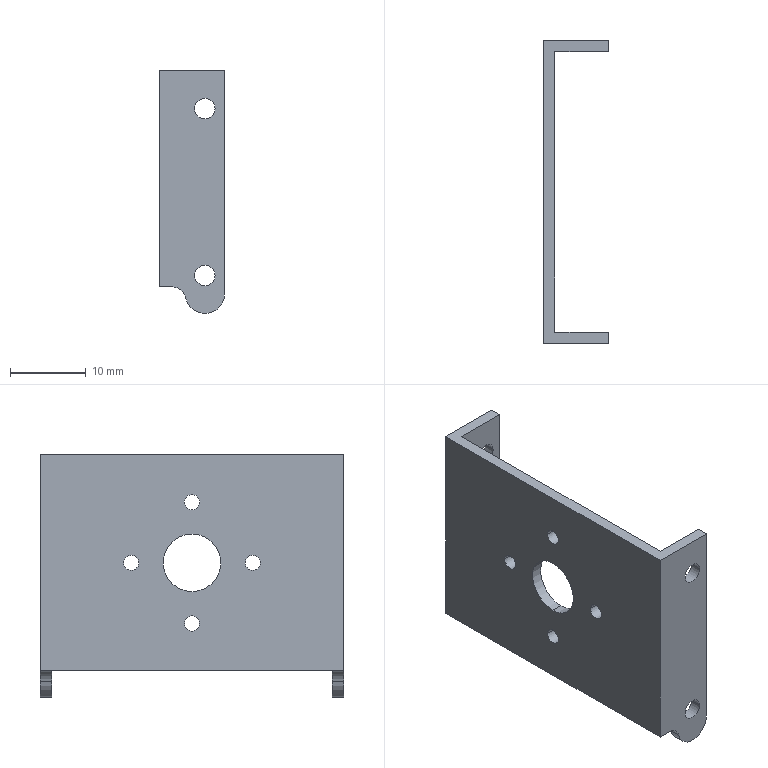Part | SolidWorks | features BaseBody 1 | 1 solid | 32 faces | box 8.6 x 40 x 32 mm | volume 2244 mm3 | cylinder 22 | plane 10 | commonest cylinder face diameters 2 x8 2.7 x8 3.485 x2 5.2 x2 7.6 x2
STEP:
#1=CARTESIAN_POINT('',(0.,19.,9.743));
#2=VERTEX_POINT('',#1);
#3=CARTESIAN_POINT('',(0.,21.,9.743));
#4=VERTEX_POINT('',#3);
#5=CARTESIAN_POINT('',(0.,20.,9.743));
#6=DIRECTION('',(1.,0.,0.));
#7=DIRECTION('',(0.,0.,1.));
#8=AXIS2_PLACEMENT_3D('',#5,#6,#7);
#9=CIRCLE('',#8,1.);
#10=EDGE_CURVE('',#2,#4,#9,.T.);
#11=ORIENTED_EDGE('',*,*,#10,.F.);
#12=CARTESIAN_POINT('',(1.5,19.,9.743));
#13=VERTEX_POINT('',#12);
#14=CARTESIAN_POINT('',(0.,19.,9.743));
#15=DIRECTION('',(1.,0.,0.));
#16=VECTOR('',#15,1000.);
#17=LINE('',#14,#16);
#18=EDGE_CURVE('',#2,#13,#17,.T.);
#19=ORIENTED_EDGE('',*,*,#18,.T.);
#20=CARTESIAN_POINT('',(1.5,21.,9.743));
#21=VERTEX_POINT('',#20);
#22=CARTESIAN_POINT('',(1.5,20.,9.743));
#23=DIRECTION('',(1.,0.,0.));
#24=DIRECTION('',(0.,0.,1.));
#25=AXIS2_PLACEMENT_3D('',#22,#23,#24);
#26=CIRCLE('',#25,1.);
#27=EDGE_CURVE('',#13,#21,#26,.T.);
#28=ORIENTED_EDGE('',*,*,#27,.T.);
#29=CARTESIAN_POINT('',(0.,21.,9.743));
#30=DIRECTION('',(1.,0.,0.));
#31=VECTOR('',#30,1000.);
#32=LINE('',#29,#31);
#33=EDGE_CURVE('',#4,#21,#32,.T.);
#34=ORIENTED_EDGE('',*,*,#33,.F.);
#35=EDGE_LOOP('',(#11,#19,#28,#34));
#36=FACE_OUTER_BOUND('',#35,.T.);
#37=CARTESIAN_POINT('',(0.,20.,9.743));
#38=DIRECTION('',(1.,0.,0.));
#39=DIRECTION('',(0.,1.,0.));
#40=AXIS2_PLACEMENT_3D('',#37,#38,#39);
#41=CYLINDRICAL_SURFACE('',#40,1.);
#42=ADVANCED_FACE('',(#36),#41,.F.);
#43=CARTESIAN_POINT('',(0.,11.,1.743));
#44=VERTEX_POINT('',#43);
#45=CARTESIAN_POINT('',(0.,13.,1.743));
#46=VERTEX_POINT('',#45);
#47=CARTESIAN_POINT('',(0.,12.,1.743));
#48=DIRECTION('',(1.,0.,0.));
#49=DIRECTION('',(0.,-1.,0.));
#50=AXIS2_PLACEMENT_3D('',#47,#48,#49);
#51=CIRCLE('',#50,1.);
#52=EDGE_CURVE('',#44,#46,#51,.T.);
#53=ORIENTED_EDGE('',*,*,#52,.F.);
#54=CARTESIAN_POINT('',(1.5,11.,1.743));
#55=VERTEX_POINT('',#54);
#56=CARTESIAN_POINT('',(0.,11.,1.743));
#57=DIRECTION('',(1.,0.,0.));
#58=VECTOR('',#57,1000.);
#59=LINE('',#56,#58);
#60=EDGE_CURVE('',#44,#55,#59,.T.);
#61=ORIENTED_EDGE('',*,*,#60,.T.);
#62=CARTESIAN_POINT('',(1.5,13.,1.743));
#63=VERTEX_POINT('',#62);
#64=CARTESIAN_POINT('',(1.5,12.,1.743));
#65=DIRECTION('',(1.,0.,0.));
#66=DIRECTION('',(0.,-1.,0.));
#67=AXIS2_PLACEMENT_3D('',#64,#65,#66);
#68=CIRCLE('',#67,1.);
#69=EDGE_CURVE('',#55,#63,#68,.T.);
#70=ORIENTED_EDGE('',*,*,#69,.T.);
#71=CARTESIAN_POINT('',(0.,13.,1.743));
#72=DIRECTION('',(1.,0.,0.));
#73=VECTOR('',#72,1000.);
#74=LINE('',#71,#73);
#75=EDGE_CURVE('',#46,#63,#74,.T.);
#76=ORIENTED_EDGE('',*,*,#75,.F.);
#77=EDGE_LOOP('',(#53,#61,#70,#76));
#78=FACE_OUTER_BOUND('',#77,.T.);
#79=CARTESIAN_POINT('',(0.,12.,1.743));
#80=DIRECTION('',(1.,0.,0.));
#81=DIRECTION('',(0.,1.,0.));
#82=AXIS2_PLACEMENT_3D('',#79,#80,#81);
#83=CYLINDRICAL_SURFACE('',#82,1.);
#84=ADVANCED_FACE('',(#78),#83,.F.);
#85=CARTESIAN_POINT('',(0.,19.,-6.257));
#86=VERTEX_POINT('',#85);
#87=CARTESIAN_POINT('',(0.,21.,-6.257));
#88=VERTEX_POINT('',#87);
#89=CARTESIAN_POINT('',(0.,20.,-6.257));
#90=DIRECTION('',(1.,0.,0.));
#91=DIRECTION('',(0.,0.,-1.));
#92=AXIS2_PLACEMENT_3D('',#89,#90,#91);
#93=CIRCLE('',#92,1.);
#94=EDGE_CURVE('',#86,#88,#93,.T.);
#95=ORIENTED_EDGE('',*,*,#94,.F.);
#96=CARTESIAN_POINT('',(1.5,19.,-6.257));
#97=VERTEX_POINT('',#96);
#98=CARTESIAN_POINT('',(0.,19.,-6.257));
#99=DIRECTION('',(1.,0.,0.));
#100=VECTOR('',#99,1000.);
#101=LINE('',#98,#100);
#102=EDGE_CURVE('',#86,#97,#101,.T.);
#103=ORIENTED_EDGE('',*,*,#102,.T.);
#104=CARTESIAN_POINT('',(1.5,21.,-6.257));
#105=VERTEX_POINT('',#104);
#106=CARTESIAN_POINT('',(1.5,20.,-6.257));
#107=DIRECTION('',(1.,0.,0.));
#108=DIRECTION('',(0.,0.,-1.));
#109=AXIS2_PLACEMENT_3D('',#106,#107,#108);
#110=CIRCLE('',#109,1.);
#111=EDGE_CURVE('',#97,#105,#110,.T.);
#112=ORIENTED_EDGE('',*,*,#111,.T.);
#113=CARTESIAN_POINT('',(0.,21.,-6.257));
#114=DIRECTION('',(1.,0.,0.));
#115=VECTOR('',#114,1000.);
#116=LINE('',#113,#115);
#117=EDGE_CURVE('',#88,#105,#116,.T.);
#118=ORIENTED_EDGE('',*,*,#117,.F.);
#119=EDGE_LOOP('',(#95,#103,#112,#118));
#120=FACE_OUTER_BOUND('',#119,.T.);
#121=CARTESIAN_POINT('',(0.,20.,-6.257));
#122=DIRECTION('',(1.,0.,0.));
#123=DIRECTION('',(0.,1.,0.));
#124=AXIS2_PLACEMENT_3D('',#121,#122,#123);
#125=CYLINDRICAL_SURFACE('',#124,1.);
#126=ADVANCED_FACE('',(#120),#125,.F.);
#127=CARTESIAN_POINT('',(0.,27.,1.743));
#128=VERTEX_POINT('',#127);
#129=CARTESIAN_POINT('',(0.,29.,1.743));
#130=VERTEX_POINT('',#129);
#131=CARTESIAN_POINT('',(0.,28.,1.743));
#132=DIRECTION('',(1.,0.,0.));
#133=DIRECTION('',(0.,1.,0.));
#134=AXIS2_PLACEMENT_3D('',#131,#132,#133);
#135=CIRCLE('',#134,1.);
#136=EDGE_CURVE('',#128,#130,#135,.T.);
#137=ORIENTED_EDGE('',*,*,#136,.F.);
#138=CARTESIAN_POINT('',(1.5,27.,1.743));
#139=VERTEX_POINT('',#138);
#140=CARTESIAN_POINT('',(0.,27.,1.743));
#141=DIRECTION('',(1.,0.,0.));
#142=VECTOR('',#141,1000.);
#143=LINE('',#140,#142);
#144=EDGE_CURVE('',#128,#139,#143,.T.);
#145=ORIENTED_EDGE('',*,*,#144,.T.);
#146=CARTESIAN_POINT('',(1.5,29.,1.743));
#147=VERTEX_POINT('',#146);
#148=CARTESIAN_POINT('',(1.5,28.,1.743));
#149=DIRECTION('',(1.,0.,0.));
#150=DIRECTION('',(0.,1.,0.));
#151=AXIS2_PLACEMENT_3D('',#148,#149,#150);
#152=CIRCLE('',#151,1.);
#153=EDGE_CURVE('',#139,#147,#152,.T.);
#154=ORIENTED_EDGE('',*,*,#153,.T.);
#155=CARTESIAN_POINT('',(0.,29.,1.743));
#156=DIRECTION('',(1.,0.,0.));
#157=VECTOR('',#156,1000.);
#158=LINE('',#155,#157);
#159=EDGE_CURVE('',#130,#147,#158,.T.);
#160=ORIENTED_EDGE('',*,*,#159,.F.);
#161=EDGE_LOOP('',(#137,#145,#154,#160));
#162=FACE_OUTER_BOUND('',#161,.T.);
#163=CARTESIAN_POINT('',(0.,28.,1.743));
#164=DIRECTION('',(1.,0.,0.));
#165=DIRECTION('',(0.,1.,0.));
#166=AXIS2_PLACEMENT_3D('',#163,#164,#165);
#167=CYLINDRICAL_SURFACE('',#166,1.);
#168=ADVANCED_FACE('',(#162),#167,.F.);
#169=CARTESIAN_POINT('',(1.5,20.,-2.057));
#170=VERTEX_POINT('',#169);
#171=CARTESIAN_POINT('',(1.5,20.,5.543));
#172=VERTEX_POINT('',#171);
#173=CARTESIAN_POINT('',(1.5,20.,1.743));
#174=DIRECTION('',(-1.,0.,0.));
#175=DIRECTION('',(0.,-1.,0.));
#176=AXIS2_PLACEMENT_3D('',#173,#174,#175);
#177=CIRCLE('',#176,3.8);
#178=EDGE_CURVE('',#170,#172,#177,.T.);
#179=ORIENTED_EDGE('',*,*,#178,.F.);
#180=CARTESIAN_POINT('',(0.,20.,-2.057));
#181=VERTEX_POINT('',#180);
#182=CARTESIAN_POINT('',(8.6,20.,-2.057));
#183=DIRECTION('',(-1.,0.,0.));
#184=VECTOR('',#183,1000.);
#185=LINE('',#182,#184);
#186=EDGE_CURVE('',#170,#181,#185,.T.);
#187=ORIENTED_EDGE('',*,*,#186,.T.);
#188=CARTESIAN_POINT('',(0.,20.,5.543));
#189=VERTEX_POINT('',#188);
#190=CARTESIAN_POINT('',(0.,20.,1.743));
#191=DIRECTION('',(-1.,0.,0.));
#192=DIRECTION('',(0.,0.,1.));
#193=AXIS2_PLACEMENT_3D('',#190,#191,#192);
#194=CIRCLE('',#193,3.8);
#195=EDGE_CURVE('',#181,#189,#194,.T.);
#196=ORIENTED_EDGE('',*,*,#195,.T.);
#197=CARTESIAN_POINT('',(8.6,20.,5.543));
#198=DIRECTION('',(-1.,0.,0.));
#199=VECTOR('',#198,1000.);
#200=LINE('',#197,#199);
#201=EDGE_CURVE('',#172,#189,#200,.T.);
#202=ORIENTED_EDGE('',*,*,#201,.F.);
#203=EDGE_LOOP('',(#179,#187,#196,#202));
#204=FACE_OUTER_BOUND('',#203,.T.);
#205=CARTESIAN_POINT('',(8.6,20.,1.743));
#206=DIRECTION('',(-1.,0.,0.));
#207=DIRECTION('',(0.,0.,1.));
#208=AXIS2_PLACEMENT_3D('',#205,#206,#207);
#209=CYLINDRICAL_SURFACE('',#208,3.8);
#210=ADVANCED_FACE('',(#204),#209,.F.);
#211=CARTESIAN_POINT('',(7.35,0.,11.));
#212=VERTEX_POINT('',#211);
#213=CARTESIAN_POINT('',(4.65,0.,11.));
#214=VERTEX_POINT('',#213);
#215=CARTESIAN_POINT('',(6.,0.,11.));
#216=DIRECTION('',(0.,1.,0.));
#217=DIRECTION('',(-1.,0.,0.));
#218=AXIS2_PLACEMENT_3D('',#215,#216,#217);
#219=CIRCLE('',#218,1.35);
#220=EDGE_CURVE('',#212,#214,#219,.T.);
#221=ORIENTED_EDGE('',*,*,#220,.F.);
#222=CARTESIAN_POINT('',(7.35,1.5,11.));
#223=VERTEX_POINT('',#222);
#224=CARTESIAN_POINT('',(7.35,0.,11.));
#225=DIRECTION('',(0.,1.,0.));
#226=VECTOR('',#225,1000.);
#227=LINE('',#224,#226);
#228=EDGE_CURVE('',#212,#223,#227,.T.);
#229=ORIENTED_EDGE('',*,*,#228,.T.);
#230=CARTESIAN_POINT('',(4.65,1.5,11.));
#231=VERTEX_POINT('',#230);
#232=CARTESIAN_POINT('',(6.,1.5,11.));
#233=DIRECTION('',(0.,-1.,0.));
#234=DIRECTION('',(0.,0.,-1.));
#235=AXIS2_PLACEMENT_3D('',#232,#233,#234);
#236=CIRCLE('',#235,1.35);
#237=EDGE_CURVE('',#231,#223,#236,.T.);
#238=ORIENTED_EDGE('',*,*,#237,.F.);
#239=CARTESIAN_POINT('',(4.65,0.,11.));
#240=DIRECTION('',(0.,1.,0.));
#241=VECTOR('',#240,1000.);
#242=LINE('',#239,#241);
#243=EDGE_CURVE('',#214,#231,#242,.T.);
#244=ORIENTED_EDGE('',*,*,#243,.F.);
#245=EDGE_LOOP('',(#221,#229,#238,#244));
#246=FACE_OUTER_BOUND('',#245,.T.);
#247=CARTESIAN_POINT('',(6.,0.,11.));
#248=DIRECTION('',(0.,1.,0.));
#249=DIRECTION('',(-1.,0.,0.));
#250=AXIS2_PLACEMENT_3D('',#247,#248,#249);
#251=CYLINDRICAL_SURFACE('',#250,1.35);
#252=ADVANCED_FACE('',(#246),#251,.F.);
#253=CARTESIAN_POINT('',(7.35,38.5,11.));
#254=VERTEX_POINT('',#253);
#255=CARTESIAN_POINT('',(4.65,38.5,11.));
#256=VERTEX_POINT('',#255);
#257=CARTESIAN_POINT('',(6.,38.5,11.));
#258=DIRECTION('',(0.,1.,0.));
#259=DIRECTION('',(0.,0.,1.));
#260=AXIS2_PLACEMENT_3D('',#257,#258,#259);
#261=CIRCLE('',#260,1.35);
#262=EDGE_CURVE('',#254,#256,#261,.T.);
#263=ORIENTED_EDGE('',*,*,#262,.F.);
#264=CARTESIAN_POINT('',(7.35,40.,11.));
#265=VERTEX_POINT('',#264);
#266=CARTESIAN_POINT('',(7.35,0.,11.));
#267=DIRECTION('',(0.,1.,0.));
#268=VECTOR('',#267,1000.);
#269=LINE('',#266,#268);
#270=EDGE_CURVE('',#254,#265,#269,.T.);
#271=ORIENTED_EDGE('',*,*,#270,.T.);
#272=CARTESIAN_POINT('',(4.65,40.,11.));
#273=VERTEX_POINT('',#272);
#274=CARTESIAN_POINT('',(6.,40.,11.));
#275=DIRECTION('',(0.,1.,0.));
#276=DIRECTION('',(-1.,0.,0.));
#277=AXIS2_PLACEMENT_3D('',#274,#275,#276);
#278=CIRCLE('',#277,1.35);
#279=EDGE_CURVE('',#265,#273,#278,.T.);
#280=ORIENTED_EDGE('',*,*,#279,.T.);
#281=CARTESIAN_POINT('',(4.65,0.,11.));
#282=DIRECTION('',(0.,1.,0.));
#283=VECTOR('',#282,1000.);
#284=LINE('',#281,#283);
#285=EDGE_CURVE('',#256,#273,#284,.T.);
#286=ORIENTED_EDGE('',*,*,#285,.F.);
#287=EDGE_LOOP('',(#263,#271,#280,#286));
#288=FACE_OUTER_BOUND('',#287,.T.);
#289=CARTESIAN_POINT('',(6.,0.,11.));
#290=DIRECTION('',(0.,1.,0.));
#291=DIRECTION('',(-1.,0.,0.));
#292=AXIS2_PLACEMENT_3D('',#289,#290,#291);
#293=CYLINDRICAL_SURFACE('',#292,1.35);
#294=ADVANCED_FACE('',(#288),#293,.F.);
#295=CARTESIAN_POINT('',(7.35,0.,-11.));
#296=VERTEX_POINT('',#295);
#297=CARTESIAN_POINT('',(4.65,0.,-11.));
#298=VERTEX_POINT('',#297);
#299=CARTESIAN_POINT('',(6.,0.,-11.));
#300=DIRECTION('',(0.,1.,0.));
#301=DIRECTION('',(-1.,0.,0.));
#302=AXIS2_PLACEMENT_3D('',#299,#300,#301);
#303=CIRCLE('',#302,1.35);
#304=EDGE_CURVE('',#296,#298,#303,.T.);
#305=ORIENTED_EDGE('',*,*,#304,.F.);
#306=CARTESIAN_POINT('',(7.35,1.5,-11.));
#307=VERTEX_POINT('',#306);
#308=CARTESIAN_POINT('',(7.35,0.,-11.));
#309=DIRECTION('',(0.,1.,0.));
#310=VECTOR('',#309,1000.);
#311=LINE('',#308,#310);
#312=EDGE_CURVE('',#296,#307,#311,.T.);
#313=ORIENTED_EDGE('',*,*,#312,.T.);
#314=CARTESIAN_POINT('',(4.65,1.5,-11.));
#315=VERTEX_POINT('',#314);
#316=CARTESIAN_POINT('',(6.,1.5,-11.));
#317=DIRECTION('',(0.,-1.,0.));
#318=DIRECTION('',(0.,0.,-1.));
#319=AXIS2_PLACEMENT_3D('',#316,#317,#318);
#320=CIRCLE('',#319,1.35);
#321=EDGE_CURVE('',#315,#307,#320,.T.);
#322=ORIENTED_EDGE('',*,*,#321,.F.);
#323=CARTESIAN_POINT('',(4.65,0.,-11.));
#324=DIRECTION('',(0.,1.,0.));
#325=VECTOR('',#324,1000.);
#326=LINE('',#323,#325);
#327=EDGE_CURVE('',#298,#315,#326,.T.);
#328=ORIENTED_EDGE('',*,*,#327,.F.);
#329=EDGE_LOOP('',(#305,#313,#322,#328));
#330=FACE_OUTER_BOUND('',#329,.T.);
#331=CARTESIAN_POINT('',(6.,0.,-11.));
#332=DIRECTION('',(0.,1.,0.));
#333=DIRECTION('',(-1.,0.,0.));
#334=AXIS2_PLACEMENT_3D('',#331,#332,#333);
#335=CYLINDRICAL_SURFACE('',#334,1.35);
#336=ADVANCED_FACE('',(#330),#335,.F.);
#337=CARTESIAN_POINT('',(7.35,38.5,-11.));
#338=VERTEX_POINT('',#337);
#339=CARTESIAN_POINT('',(4.65,38.5,-11.));
#340=VERTEX_POINT('',#339);
#341=CARTESIAN_POINT('',(6.,38.5,-11.));
#342=DIRECTION('',(0.,1.,0.));
#343=DIRECTION('',(0.,0.,1.));
#344=AXIS2_PLACEMENT_3D('',#341,#342,#343);
#345=CIRCLE('',#344,1.35);
#346=EDGE_CURVE('',#338,#340,#345,.T.);
#347=ORIENTED_EDGE('',*,*,#346,.F.);
#348=CARTESIAN_POINT('',(7.35,40.,-11.));
#349=VERTEX_POINT('',#348);
#350=CARTESIAN_POINT('',(7.35,0.,-11.));
#351=DIRECTION('',(0.,1.,0.));
#352=VECTOR('',#351,1000.);
#353=LINE('',#350,#352);
#354=EDGE_CURVE('',#338,#349,#353,.T.);
#355=ORIENTED_EDGE('',*,*,#354,.T.);
#356=CARTESIAN_POINT('',(4.65,40.,-11.));
#357=VERTEX_POINT('',#356);
#358=CARTESIAN_POINT('',(6.,40.,-11.));
#359=DIRECTION('',(0.,1.,0.));
#360=DIRECTION('',(-1.,0.,0.));
#361=AXIS2_PLACEMENT_3D('',#358,#359,#360);
#362=CIRCLE('',#361,1.35);
#363=EDGE_CURVE('',#349,#357,#362,.T.);
#364=ORIENTED_EDGE('',*,*,#363,.T.);
#365=CARTESIAN_POINT('',(4.65,0.,-11.));
#366=DIRECTION('',(0.,1.,0.));
#367=VECTOR('',#366,1000.);
#368=LINE('',#365,#367);
#369=EDGE_CURVE('',#340,#357,#368,.T.);
#370=ORIENTED_EDGE('',*,*,#369,.F.);
#371=EDGE_LOOP('',(#347,#355,#364,#370));
#372=FACE_OUTER_BOUND('',#371,.T.);
#373=CARTESIAN_POINT('',(6.,0.,-11.));
#374=DIRECTION('',(0.,1.,0.));
#375=DIRECTION('',(-1.,0.,0.));
#376=AXIS2_PLACEMENT_3D('',#373,#374,#375);
#377=CYLINDRICAL_SURFACE('',#376,1.35);
#378=ADVANCED_FACE('',(#372),#377,.F.);
#379=CARTESIAN_POINT('',(6.,0.,11.));
#380=DIRECTION('',(0.,1.,0.));
#381=DIRECTION('',(-1.,0.,0.));
#382=AXIS2_PLACEMENT_3D('',#379,#380,#381);
#383=CIRCLE('',#382,1.35);
#384=EDGE_CURVE('',#214,#212,#383,.T.);
#385=ORIENTED_EDGE('',*,*,#384,.T.);
#386=ORIENTED_EDGE('',*,*,#220,.T.);
#387=EDGE_LOOP('',(#385,#386));
#388=FACE_BOUND('',#387,.T.);
#389=CARTESIAN_POINT('',(6.,0.,-11.));
#390=DIRECTION('',(0.,1.,0.));
#391=DIRECTION('',(-1.,0.,0.));
#392=AXIS2_PLACEMENT_3D('',#389,#390,#391);
#393=CIRCLE('',#392,1.35);
#394=EDGE_CURVE('',#298,#296,#393,.T.);
#395=ORIENTED_EDGE('',*,*,#394,.T.);
#396=ORIENTED_EDGE('',*,*,#304,.T.);
#397=EDGE_LOOP('',(#395,#396));
#398=FACE_BOUND('',#397,.T.);
#399=CARTESIAN_POINT('',(8.6,0.,-13.4));
#400=VERTEX_POINT('',#399);
#401=CARTESIAN_POINT('',(3.451,0.,-13.913));
#402=VERTEX_POINT('',#401);
#403=CARTESIAN_POINT('',(6.,0.,-13.4));
#404=DIRECTION('',(0.,1.,0.));
#405=DIRECTION('',(0.,0.,1.));
#406=AXIS2_PLACEMENT_3D('',#403,#404,#405);
#407=CIRCLE('',#406,2.6);
#408=EDGE_CURVE('',#400,#402,#407,.T.);
#409=ORIENTED_EDGE('',*,*,#408,.F.);
#410=CARTESIAN_POINT('',(8.6,0.,16.));
#411=VERTEX_POINT('',#410);
#412=CARTESIAN_POINT('',(8.6,0.,16.));
#413=DIRECTION('',(0.,0.,-1.));
#414=VECTOR('',#413,1000.);
#415=LINE('',#412,#414);
#416=EDGE_CURVE('',#411,#400,#415,.T.);
#417=ORIENTED_EDGE('',*,*,#416,.F.);
#418=CARTESIAN_POINT('',(0.,0.,16.));
#419=VERTEX_POINT('',#418);
#420=CARTESIAN_POINT('',(8.6,0.,16.));
#421=DIRECTION('',(1.,0.,0.));
#422=VECTOR('',#421,1000.);
#423=LINE('',#420,#422);
#424=EDGE_CURVE('',#419,#411,#423,.T.);
#425=ORIENTED_EDGE('',*,*,#424,.F.);
#426=CARTESIAN_POINT('',(0.,0.,-12.515));
#427=VERTEX_POINT('',#426);
#428=CARTESIAN_POINT('',(0.,0.,16.));
#429=DIRECTION('',(0.,0.,-1.));
#430=VECTOR('',#429,1000.);
#431=LINE('',#428,#430);
#432=EDGE_CURVE('',#419,#427,#431,.T.);
#433=ORIENTED_EDGE('',*,*,#432,.T.);
#434=CARTESIAN_POINT('',(1.743,0.,-12.515));
#435=VERTEX_POINT('',#434);
#436=CARTESIAN_POINT('',(0.,0.,-12.515));
#437=DIRECTION('',(-1.,0.,0.));
#438=VECTOR('',#437,1000.);
#439=LINE('',#436,#438);
#440=EDGE_CURVE('',#435,#427,#439,.T.);
#441=ORIENTED_EDGE('',*,*,#440,.F.);
#442=CARTESIAN_POINT('',(1.743,0.,-14.257));
#443=DIRECTION('',(0.,1.,0.));
#444=DIRECTION('',(0.,0.,1.));
#445=AXIS2_PLACEMENT_3D('',#442,#443,#444);
#446=CIRCLE('',#445,1.743);
#447=EDGE_CURVE('',#435,#402,#446,.T.);
#448=ORIENTED_EDGE('',*,*,#447,.T.);
#449=EDGE_LOOP('',(#409,#417,#425,#433,#441,#448));
#450=FACE_OUTER_BOUND('',#449,.T.);
#451=CARTESIAN_POINT('',(8.6,0.,16.));
#452=DIRECTION('',(0.,1.,0.));
#453=DIRECTION('',(-1.,0.,0.));
#454=AXIS2_PLACEMENT_3D('',#451,#452,#453);
#455=PLANE('',#454);
#456=ADVANCED_FACE('',(#388,#398,#450),#455,.F.);
#457=ORIENTED_EDGE('',*,*,#237,.T.);
#458=CARTESIAN_POINT('',(6.,1.5,11.));
#459=DIRECTION('',(0.,-1.,0.));
#460=DIRECTION('',(0.,0.,-1.));
#461=AXIS2_PLACEMENT_3D('',#458,#459,#460);
#462=CIRCLE('',#461,1.35);
#463=EDGE_CURVE('',#223,#231,#462,.T.);
#464=ORIENTED_EDGE('',*,*,#463,.T.);
#465=EDGE_LOOP('',(#457,#464));
#466=FACE_BOUND('',#465,.T.);
#467=ORIENTED_EDGE('',*,*,#321,.T.);
#468=CARTESIAN_POINT('',(6.,1.5,-11.));
#469=DIRECTION('',(0.,-1.,0.));
#470=DIRECTION('',(0.,0.,-1.));
#471=AXIS2_PLACEMENT_3D('',#468,#469,#470);
#472=CIRCLE('',#471,1.35);
#473=EDGE_CURVE('',#307,#315,#472,.T.);
#474=ORIENTED_EDGE('',*,*,#473,.T.);
#475=EDGE_LOOP('',(#467,#474));
#476=FACE_BOUND('',#475,.T.);
#477=CARTESIAN_POINT('',(8.6,1.5,16.));
#478=VERTEX_POINT('',#477);
#479=CARTESIAN_POINT('',(8.6,1.5,-13.4));
#480=VERTEX_POINT('',#479);
#481=CARTESIAN_POINT('',(8.6,1.5,16.));
#482=DIRECTION('',(0.,0.,-1.));
#483=VECTOR('',#482,1000.);
#484=LINE('',#481,#483);
#485=EDGE_CURVE('',#478,#480,#484,.T.);
#486=ORIENTED_EDGE('',*,*,#485,.T.);
#487=CARTESIAN_POINT('',(3.451,1.5,-13.913));
#488=VERTEX_POINT('',#487);
#489=CARTESIAN_POINT('',(6.,1.5,-13.4));
#490=DIRECTION('',(0.,-1.,0.));
#491=DIRECTION('',(0.,0.,-1.));
#492=AXIS2_PLACEMENT_3D('',#489,#490,#491);
#493=CIRCLE('',#492,2.6);
#494=EDGE_CURVE('',#488,#480,#493,.T.);
#495=ORIENTED_EDGE('',*,*,#494,.F.);
#496=CARTESIAN_POINT('',(1.743,1.5,-12.515));
#497=VERTEX_POINT('',#496);
#498=CARTESIAN_POINT('',(1.743,1.5,-14.257));
#499=DIRECTION('',(0.,-1.,0.));
#500=DIRECTION('',(0.,0.,-1.));
#501=AXIS2_PLACEMENT_3D('',#498,#499,#500);
#502=CIRCLE('',#501,1.743);
#503=EDGE_CURVE('',#488,#497,#502,.T.);
#504=ORIENTED_EDGE('',*,*,#503,.T.);
#505=CARTESIAN_POINT('',(1.5,1.5,-12.515));
#506=VERTEX_POINT('',#505);
#507=CARTESIAN_POINT('',(1.5,1.5,-12.515));
#508=DIRECTION('',(1.,0.,0.));
#509=VECTOR('',#508,1000.);
#510=LINE('',#507,#509);
#511=EDGE_CURVE('',#506,#497,#510,.T.);
#512=ORIENTED_EDGE('',*,*,#511,.F.);
#513=CARTESIAN_POINT('',(1.5,1.5,16.));
#514=VERTEX_POINT('',#513);
#515=CARTESIAN_POINT('',(1.5,1.5,16.));
#516=DIRECTION('',(0.,0.,-1.));
#517=VECTOR('',#516,1000.);
#518=LINE('',#515,#517);
#519=EDGE_CURVE('',#514,#506,#518,.T.);
#520=ORIENTED_EDGE('',*,*,#519,.F.);
#521=CARTESIAN_POINT('',(1.5,1.5,16.));
#522=DIRECTION('',(-1.,0.,0.));
#523=VECTOR('',#522,1000.);
#524=LINE('',#521,#523);
#525=EDGE_CURVE('',#478,#514,#524,.T.);
#526=ORIENTED_EDGE('',*,*,#525,.F.);
#527=EDGE_LOOP('',(#486,#495,#504,#512,#520,#526));
#528=FACE_OUTER_BOUND('',#527,.T.);
#529=CARTESIAN_POINT('',(1.5,1.5,16.));
#530=DIRECTION('',(0.,-1.,0.));
#531=DIRECTION('',(0.,0.,-1.));
#532=AXIS2_PLACEMENT_3D('',#529,#530,#531);
#533=PLANE('',#532);
#534=ADVANCED_FACE('',(#466,#476,#528),#533,.F.);
#535=CARTESIAN_POINT('',(1.5,20.,9.743));
#536=DIRECTION('',(1.,0.,0.));
#537=DIRECTION('',(0.,0.,1.));
#538=AXIS2_PLACEMENT_3D('',#535,#536,#537);
#539=CIRCLE('',#538,1.);
#540=EDGE_CURVE('',#21,#13,#539,.T.);
#541=ORIENTED_EDGE('',*,*,#540,.F.);
#542=ORIENTED_EDGE('',*,*,#27,.F.);
#543=EDGE_LOOP('',(#541,#542));
#544=FACE_BOUND('',#543,.T.);
#545=CARTESIAN_POINT('',(1.5,12.,1.743));
#546=DIRECTION('',(1.,0.,0.));
#547=DIRECTION('',(0.,-1.,0.));
#548=AXIS2_PLACEMENT_3D('',#545,#546,#547);
#549=CIRCLE('',#548,1.);
#550=EDGE_CURVE('',#63,#55,#549,.T.);
#551=ORIENTED_EDGE('',*,*,#550,.F.);
#552=ORIENTED_EDGE('',*,*,#69,.F.);
#553=EDGE_LOOP('',(#551,#552));
#554=FACE_BOUND('',#553,.T.);
#555=CARTESIAN_POINT('',(1.5,20.,-6.257));
#556=DIRECTION('',(1.,0.,0.));
#557=DIRECTION('',(0.,0.,-1.));
#558=AXIS2_PLACEMENT_3D('',#555,#556,#557);
#559=CIRCLE('',#558,1.);
#560=EDGE_CURVE('',#105,#97,#559,.T.);
#561=ORIENTED_EDGE('',*,*,#560,.F.);
#562=ORIENTED_EDGE('',*,*,#111,.F.);
#563=EDGE_LOOP('',(#561,#562));
#564=FACE_BOUND('',#563,.T.);
#565=CARTESIAN_POINT('',(1.5,28.,1.743));
#566=DIRECTION('',(1.,0.,0.));
#567=DIRECTION('',(0.,1.,0.));
#568=AXIS2_PLACEMENT_3D('',#565,#566,#567);
#569=CIRCLE('',#568,1.);
#570=EDGE_CURVE('',#147,#139,#569,.T.);
#571=ORIENTED_EDGE('',*,*,#570,.F.);
#572=ORIENTED_EDGE('',*,*,#153,.F.);
#573=EDGE_LOOP('',(#571,#572));
#574=FACE_BOUND('',#573,.T.);
#575=CARTESIAN_POINT('',(1.5,20.,1.743));
#576=DIRECTION('',(-1.,0.,0.));
#577=DIRECTION('',(0.,-1.,0.));
#578=AXIS2_PLACEMENT_3D('',#575,#576,#577);
#579=CIRCLE('',#578,3.8);
#580=EDGE_CURVE('',#172,#170,#579,.T.);
#581=ORIENTED_EDGE('',*,*,#580,.T.);
#582=ORIENTED_EDGE('',*,*,#178,.T.);
#583=EDGE_LOOP('',(#581,#582));
#584=FACE_BOUND('',#583,.T.);
#585=CARTESIAN_POINT('',(1.5,38.5,-12.515));
#586=VERTEX_POINT('',#585);
#587=CARTESIAN_POINT('',(1.5,38.5,-12.515));
#588=DIRECTION('',(0.,-1.,0.));
#589=VECTOR('',#588,1000.);
#590=LINE('',#587,#589);
#591=EDGE_CURVE('',#586,#506,#590,.T.);
#592=ORIENTED_EDGE('',*,*,#591,.F.);
#593=CARTESIAN_POINT('',(1.5,38.5,16.));
#594=VERTEX_POINT('',#593);
#595=CARTESIAN_POINT('',(1.5,38.5,16.));
#596=DIRECTION('',(0.,0.,-1.));
#597=VECTOR('',#596,1000.);
#598=LINE('',#595,#597);
#599=EDGE_CURVE('',#594,#586,#598,.T.);
#600=ORIENTED_EDGE('',*,*,#599,.F.);
#601=CARTESIAN_POINT('',(1.5,38.5,16.));
#602=DIRECTION('',(0.,1.,0.));
#603=VECTOR('',#602,1000.);
#604=LINE('',#601,#603);
#605=EDGE_CURVE('',#514,#594,#604,.T.);
#606=ORIENTED_EDGE('',*,*,#605,.F.);
#607=ORIENTED_EDGE('',*,*,#519,.T.);
#608=EDGE_LOOP('',(#592,#600,#606,#607));
#609=FACE_OUTER_BOUND('',#608,.T.);
#610=CARTESIAN_POINT('',(1.5,38.5,16.));
#611=DIRECTION('',(-1.,0.,0.));
#612=DIRECTION('',(0.,-1.,0.));
#613=AXIS2_PLACEMENT_3D('',#610,#611,#612);
#614=PLANE('',#613);
#615=ADVANCED_FACE('',(#544,#554,#564,#574,#584,#609),#614,.F.);
#616=CARTESIAN_POINT('',(6.,38.5,11.));
#617=DIRECTION('',(0.,1.,0.));
#618=DIRECTION('',(0.,0.,1.));
#619=AXIS2_PLACEMENT_3D('',#616,#617,#618);
#620=CIRCLE('',#619,1.35);
#621=EDGE_CURVE('',#256,#254,#620,.T.);
#622=ORIENTED_EDGE('',*,*,#621,.T.);
#623=ORIENTED_EDGE('',*,*,#262,.T.);
#624=EDGE_LOOP('',(#622,#623));
#625=FACE_BOUND('',#624,.T.);
#626=CARTESIAN_POINT('',(6.,38.5,-11.));
#627=DIRECTION('',(0.,1.,0.));
#628=DIRECTION('',(0.,0.,1.));
#629=AXIS2_PLACEMENT_3D('',#626,#627,#628);
#630=CIRCLE('',#629,1.35);
#631=EDGE_CURVE('',#340,#338,#630,.T.);
#632=ORIENTED_EDGE('',*,*,#631,.T.);
#633=ORIENTED_EDGE('',*,*,#346,.T.);
#634=EDGE_LOOP('',(#632,#633));
#635=FACE_BOUND('',#634,.T.);
#636=CARTESIAN_POINT('',(8.6,38.5,-13.4));
#637=VERTEX_POINT('',#636);
#638=CARTESIAN_POINT('',(3.451,38.5,-13.913));
#639=VERTEX_POINT('',#638);
#640=CARTESIAN_POINT('',(6.,38.5,-13.4));
#641=DIRECTION('',(0.,1.,0.));
#642=DIRECTION('',(0.,0.,1.));
#643=AXIS2_PLACEMENT_3D('',#640,#641,#642);
#644=CIRCLE('',#643,2.6);
#645=EDGE_CURVE('',#637,#639,#644,.T.);
#646=ORIENTED_EDGE('',*,*,#645,.F.);
#647=CARTESIAN_POINT('',(8.6,38.5,16.));
#648=VERTEX_POINT('',#647);
#649=CARTESIAN_POINT('',(8.6,38.5,16.));
#650=DIRECTION('',(0.,0.,-1.));
#651=VECTOR('',#650,1000.);
#652=LINE('',#649,#651);
#653=EDGE_CURVE('',#648,#637,#652,.T.);
#654=ORIENTED_EDGE('',*,*,#653,.F.);
#655=CARTESIAN_POINT('',(8.6,38.5,16.));
#656=DIRECTION('',(1.,0.,0.));
#657=VECTOR('',#656,1000.);
#658=LINE('',#655,#657);
#659=EDGE_CURVE('',#594,#648,#658,.T.);
#660=ORIENTED_EDGE('',*,*,#659,.F.);
#661=ORIENTED_EDGE('',*,*,#599,.T.);
#662=CARTESIAN_POINT('',(1.743,38.5,-12.515));
#663=VERTEX_POINT('',#662);
#664=CARTESIAN_POINT('',(8.6,38.5,-12.515));
#665=DIRECTION('',(-1.,0.,0.));
#666=VECTOR('',#665,1000.);
#667=LINE('',#664,#666);
#668=EDGE_CURVE('',#663,#586,#667,.T.);
#669=ORIENTED_EDGE('',*,*,#668,.F.);
#670=CARTESIAN_POINT('',(1.743,38.5,-14.257));
#671=DIRECTION('',(0.,1.,0.));
#672=DIRECTION('',(0.,0.,1.));
#673=AXIS2_PLACEMENT_3D('',#670,#671,#672);
#674=CIRCLE('',#673,1.743);
#675=EDGE_CURVE('',#663,#639,#674,.T.);
#676=ORIENTED_EDGE('',*,*,#675,.T.);
#677=EDGE_LOOP('',(#646,#654,#660,#661,#669,#676));
#678=FACE_OUTER_BOUND('',#677,.T.);
#679=CARTESIAN_POINT('',(8.6,38.5,16.));
#680=DIRECTION('',(0.,1.,0.));
#681=DIRECTION('',(0.,0.,1.));
#682=AXIS2_PLACEMENT_3D('',#679,#680,#681);
#683=PLANE('',#682);
#684=ADVANCED_FACE('',(#625,#635,#678),#683,.F.);
#685=CARTESIAN_POINT('',(6.,40.,11.));
#686=DIRECTION('',(0.,1.,0.));
#687=DIRECTION('',(-1.,0.,0.));
#688=AXIS2_PLACEMENT_3D('',#685,#686,#687);
#689=CIRCLE('',#688,1.35);
#690=EDGE_CURVE('',#273,#265,#689,.T.);
#691=ORIENTED_EDGE('',*,*,#690,.F.);
#692=ORIENTED_EDGE('',*,*,#279,.F.);
#693=EDGE_LOOP('',(#691,#692));
#694=FACE_BOUND('',#693,.T.);
#695=CARTESIAN_POINT('',(6.,40.,-11.));
#696=DIRECTION('',(0.,1.,0.));
#697=DIRECTION('',(-1.,0.,0.));
#698=AXIS2_PLACEMENT_3D('',#695,#696,#697);
#699=CIRCLE('',#698,1.35);
#700=EDGE_CURVE('',#357,#349,#699,.T.);
#701=ORIENTED_EDGE('',*,*,#700,.F.);
#702=ORIENTED_EDGE('',*,*,#363,.F.);
#703=EDGE_LOOP('',(#701,#702));
#704=FACE_BOUND('',#703,.T.);
#705=CARTESIAN_POINT('',(8.6,40.,-13.4));
#706=VERTEX_POINT('',#705);
#707=CARTESIAN_POINT('',(3.451,40.,-13.913));
#708=VERTEX_POINT('',#707);
#709=CARTESIAN_POINT('',(6.,40.,-13.4));
#710=DIRECTION('',(0.,1.,0.));
#711=DIRECTION('',(0.,0.,1.));
#712=AXIS2_PLACEMENT_3D('',#709,#710,#711);
#713=CIRCLE('',#712,2.6);
#714=EDGE_CURVE('',#706,#708,#713,.T.);
#715=ORIENTED_EDGE('',*,*,#714,.T.);
#716=CARTESIAN_POINT('',(1.743,40.,-12.515));
#717=VERTEX_POINT('',#716);
#718=CARTESIAN_POINT('',(1.743,40.,-14.257));
#719=DIRECTION('',(0.,1.,0.));
#720=DIRECTION('',(0.,0.,1.));
#721=AXIS2_PLACEMENT_3D('',#718,#719,#720);
#722=CIRCLE('',#721,1.743);
#723=EDGE_CURVE('',#717,#708,#722,.T.);
#724=ORIENTED_EDGE('',*,*,#723,.F.);
#725=CARTESIAN_POINT('',(0.,40.,-12.515));
#726=VERTEX_POINT('',#725);
#727=CARTESIAN_POINT('',(0.,40.,-12.515));
#728=DIRECTION('',(-1.,0.,0.));
#729=VECTOR('',#728,1000.);
#730=LINE('',#727,#729);
#731=EDGE_CURVE('',#717,#726,#730,.T.);
#732=ORIENTED_EDGE('',*,*,#731,.T.);
#733=CARTESIAN_POINT('',(0.,40.,16.));
#734=VERTEX_POINT('',#733);
#735=CARTESIAN_POINT('',(0.,40.,16.));
#736=DIRECTION('',(0.,0.,-1.));
#737=VECTOR('',#736,1000.);
#738=LINE('',#735,#737);
#739=EDGE_CURVE('',#734,#726,#738,.T.);
#740=ORIENTED_EDGE('',*,*,#739,.F.);
#741=CARTESIAN_POINT('',(8.6,40.,16.));
#742=VERTEX_POINT('',#741);
#743=CARTESIAN_POINT('',(0.,40.,16.));
#744=DIRECTION('',(-1.,0.,0.));
#745=VECTOR('',#744,1000.);
#746=LINE('',#743,#745);
#747=EDGE_CURVE('',#742,#734,#746,.T.);
#748=ORIENTED_EDGE('',*,*,#747,.F.);
#749=CARTESIAN_POINT('',(8.6,40.,16.));
#750=DIRECTION('',(0.,0.,-1.));
#751=VECTOR('',#750,1000.);
#752=LINE('',#749,#751);
#753=EDGE_CURVE('',#742,#706,#752,.T.);
#754=ORIENTED_EDGE('',*,*,#753,.T.);
#755=EDGE_LOOP('',(#715,#724,#732,#740,#748,#754));
#756=FACE_OUTER_BOUND('',#755,.T.);
#757=CARTESIAN_POINT('',(0.,40.,16.));
#758=DIRECTION('',(0.,-1.,0.));
#759=DIRECTION('',(0.,0.,-1.));
#760=AXIS2_PLACEMENT_3D('',#757,#758,#759);
#761=PLANE('',#760);
#762=ADVANCED_FACE('',(#694,#704,#756),#761,.F.);
#763=CARTESIAN_POINT('',(0.,20.,9.743));
#764=DIRECTION('',(1.,0.,0.));
#765=DIRECTION('',(0.,0.,1.));
#766=AXIS2_PLACEMENT_3D('',#763,#764,#765);
#767=CIRCLE('',#766,1.);
#768=EDGE_CURVE('',#4,#2,#767,.T.);
#769=ORIENTED_EDGE('',*,*,#768,.T.);
#770=ORIENTED_EDGE('',*,*,#10,.T.);
#771=EDGE_LOOP('',(#769,#770));
#772=FACE_BOUND('',#771,.T.);
#773=CARTESIAN_POINT('',(0.,12.,1.743));
#774=DIRECTION('',(1.,0.,0.));
#775=DIRECTION('',(0.,-1.,0.));
#776=AXIS2_PLACEMENT_3D('',#773,#774,#775);
#777=CIRCLE('',#776,1.);
#778=EDGE_CURVE('',#46,#44,#777,.T.);
#779=ORIENTED_EDGE('',*,*,#778,.T.);
#780=ORIENTED_EDGE('',*,*,#52,.T.);
#781=EDGE_LOOP('',(#779,#780));
#782=FACE_BOUND('',#781,.T.);
#783=CARTESIAN_POINT('',(0.,20.,-6.257));
#784=DIRECTION('',(1.,0.,0.));
#785=DIRECTION('',(0.,0.,-1.));
#786=AXIS2_PLACEMENT_3D('',#783,#784,#785);
#787=CIRCLE('',#786,1.);
#788=EDGE_CURVE('',#88,#86,#787,.T.);
#789=ORIENTED_EDGE('',*,*,#788,.T.);
#790=ORIENTED_EDGE('',*,*,#94,.T.);
#791=EDGE_LOOP('',(#789,#790));
#792=FACE_BOUND('',#791,.T.);
#793=CARTESIAN_POINT('',(0.,28.,1.743));
#794=DIRECTION('',(1.,0.,0.));
#795=DIRECTION('',(0.,1.,0.));
#796=AXIS2_PLACEMENT_3D('',#793,#794,#795);
#797=CIRCLE('',#796,1.);
#798=EDGE_CURVE('',#130,#128,#797,.T.);
#799=ORIENTED_EDGE('',*,*,#798,.T.);
#800=ORIENTED_EDGE('',*,*,#136,.T.);
#801=EDGE_LOOP('',(#799,#800));
#802=FACE_BOUND('',#801,.T.);
#803=CARTESIAN_POINT('',(0.,20.,1.743));
#804=DIRECTION('',(-1.,0.,0.));
#805=DIRECTION('',(0.,0.,1.));
#806=AXIS2_PLACEMENT_3D('',#803,#804,#805);
#807=CIRCLE('',#806,3.8);
#808=EDGE_CURVE('',#189,#181,#807,.T.);
#809=ORIENTED_EDGE('',*,*,#808,.F.);
#810=ORIENTED_EDGE('',*,*,#195,.F.);
#811=EDGE_LOOP('',(#809,#810));
#812=FACE_BOUND('',#811,.T.);
#813=CARTESIAN_POINT('',(0.,0.,-12.515));
#814=DIRECTION('',(0.,1.,0.));
#815=VECTOR('',#814,1000.);
#816=LINE('',#813,#815);
#817=EDGE_CURVE('',#427,#726,#816,.T.);
#818=ORIENTED_EDGE('',*,*,#817,.F.);
#819=ORIENTED_EDGE('',*,*,#432,.F.);
#820=CARTESIAN_POINT('',(0.,0.,16.));
#821=DIRECTION('',(0.,-1.,0.));
#822=VECTOR('',#821,1000.);
#823=LINE('',#820,#822);
#824=EDGE_CURVE('',#734,#419,#823,.T.);
#825=ORIENTED_EDGE('',*,*,#824,.F.);
#826=ORIENTED_EDGE('',*,*,#739,.T.);
#827=EDGE_LOOP('',(#818,#819,#825,#826));
#828=FACE_OUTER_BOUND('',#827,.T.);
#829=CARTESIAN_POINT('',(0.,0.,16.));
#830=DIRECTION('',(1.,0.,0.));
#831=DIRECTION('',(0.,0.,-1.));
#832=AXIS2_PLACEMENT_3D('',#829,#830,#831);
#833=PLANE('',#832);
#834=ADVANCED_FACE('',(#772,#782,#792,#802,#812,#828),#833,.F.);
#835=ORIENTED_EDGE('',*,*,#416,.T.);
#836=CARTESIAN_POINT('',(8.6,0.,-13.4));
#837=DIRECTION('',(0.,1.,0.));
#838=VECTOR('',#837,1000.);
#839=LINE('',#836,#838);
#840=EDGE_CURVE('',#400,#480,#839,.T.);
#841=ORIENTED_EDGE('',*,*,#840,.T.);
#842=ORIENTED_EDGE('',*,*,#485,.F.);
#843=CARTESIAN_POINT('',(8.6,1.5,16.));
#844=DIRECTION('',(0.,1.,0.));
#845=VECTOR('',#844,1000.);
#846=LINE('',#843,#845);
#847=EDGE_CURVE('',#411,#478,#846,.T.);
#848=ORIENTED_EDGE('',*,*,#847,.F.);
#849=EDGE_LOOP('',(#835,#841,#842,#848));
#850=FACE_OUTER_BOUND('',#849,.T.);
#851=CARTESIAN_POINT('',(8.6,1.5,16.));
#852=DIRECTION('',(-1.,0.,0.));
#853=DIRECTION('',(0.,0.,1.));
#854=AXIS2_PLACEMENT_3D('',#851,#852,#853);
#855=PLANE('',#854);
#856=ADVANCED_FACE('',(#850),#855,.F.);
#857=ORIENTED_EDGE('',*,*,#653,.T.);
#858=CARTESIAN_POINT('',(8.6,0.,-13.4));
#859=DIRECTION('',(0.,1.,0.));
#860=VECTOR('',#859,1000.);
#861=LINE('',#858,#860);
#862=EDGE_CURVE('',#637,#706,#861,.T.);
#863=ORIENTED_EDGE('',*,*,#862,.T.);
#864=ORIENTED_EDGE('',*,*,#753,.F.);
#865=CARTESIAN_POINT('',(8.6,40.,16.));
#866=DIRECTION('',(0.,1.,0.));
#867=VECTOR('',#866,1000.);
#868=LINE('',#865,#867);
#869=EDGE_CURVE('',#648,#742,#868,.T.);
#870=ORIENTED_EDGE('',*,*,#869,.F.);
#871=EDGE_LOOP('',(#857,#863,#864,#870));
#872=FACE_OUTER_BOUND('',#871,.T.);
#873=CARTESIAN_POINT('',(8.6,40.,16.));
#874=DIRECTION('',(-1.,0.,0.));
#875=DIRECTION('',(0.,0.,1.));
#876=AXIS2_PLACEMENT_3D('',#873,#874,#875);
#877=PLANE('',#876);
#878=ADVANCED_FACE('',(#872),#877,.F.);
#879=ORIENTED_EDGE('',*,*,#424,.T.);
#880=ORIENTED_EDGE('',*,*,#847,.T.);
#881=ORIENTED_EDGE('',*,*,#525,.T.);
#882=ORIENTED_EDGE('',*,*,#605,.T.);
#883=ORIENTED_EDGE('',*,*,#659,.T.);
#884=ORIENTED_EDGE('',*,*,#869,.T.);
#885=ORIENTED_EDGE('',*,*,#747,.T.);
#886=ORIENTED_EDGE('',*,*,#824,.T.);
#887=EDGE_LOOP('',(#879,#880,#881,#882,#883,#884,#885,#886));
#888=FACE_OUTER_BOUND('',#887,.T.);
#889=CARTESIAN_POINT('',(0.,0.,16.));
#890=DIRECTION('',(0.,0.,-1.));
#891=DIRECTION('',(-1.,0.,0.));
#892=AXIS2_PLACEMENT_3D('',#889,#890,#891);
#893=PLANE('',#892);
#894=ADVANCED_FACE('',(#888),#893,.F.);
#895=ORIENTED_EDGE('',*,*,#354,.F.);
#896=ORIENTED_EDGE('',*,*,#631,.F.);
#897=ORIENTED_EDGE('',*,*,#369,.T.);
#898=ORIENTED_EDGE('',*,*,#700,.T.);
#899=EDGE_LOOP('',(#895,#896,#897,#898));
#900=FACE_OUTER_BOUND('',#899,.T.);
#901=CARTESIAN_POINT('',(6.,0.,-11.));
#902=DIRECTION('',(0.,1.,0.));
#903=DIRECTION('',(-1.,0.,0.));
#904=AXIS2_PLACEMENT_3D('',#901,#902,#903);
#905=CYLINDRICAL_SURFACE('',#904,1.35);
#906=ADVANCED_FACE('',(#900),#905,.F.);
#907=ORIENTED_EDGE('',*,*,#312,.F.);
#908=ORIENTED_EDGE('',*,*,#394,.F.);
#909=ORIENTED_EDGE('',*,*,#327,.T.);
#910=ORIENTED_EDGE('',*,*,#473,.F.);
#911=EDGE_LOOP('',(#907,#908,#909,#910));
#912=FACE_OUTER_BOUND('',#911,.T.);
#913=CARTESIAN_POINT('',(6.,0.,-11.));
#914=DIRECTION('',(0.,1.,0.));
#915=DIRECTION('',(-1.,0.,0.));
#916=AXIS2_PLACEMENT_3D('',#913,#914,#915);
#917=CYLINDRICAL_SURFACE('',#916,1.35);
#918=ADVANCED_FACE('',(#912),#917,.F.);
#919=ORIENTED_EDGE('',*,*,#270,.F.);
#920=ORIENTED_EDGE('',*,*,#621,.F.);
#921=ORIENTED_EDGE('',*,*,#285,.T.);
#922=ORIENTED_EDGE('',*,*,#690,.T.);
#923=EDGE_LOOP('',(#919,#920,#921,#922));
#924=FACE_OUTER_BOUND('',#923,.T.);
#925=CARTESIAN_POINT('',(6.,0.,11.));
#926=DIRECTION('',(0.,1.,0.));
#927=DIRECTION('',(-1.,0.,0.));
#928=AXIS2_PLACEMENT_3D('',#925,#926,#927);
#929=CYLINDRICAL_SURFACE('',#928,1.35);
#930=ADVANCED_FACE('',(#924),#929,.F.);
#931=ORIENTED_EDGE('',*,*,#228,.F.);
#932=ORIENTED_EDGE('',*,*,#384,.F.);
#933=ORIENTED_EDGE('',*,*,#243,.T.);
#934=ORIENTED_EDGE('',*,*,#463,.F.);
#935=EDGE_LOOP('',(#931,#932,#933,#934));
#936=FACE_OUTER_BOUND('',#935,.T.);
#937=CARTESIAN_POINT('',(6.,0.,11.));
#938=DIRECTION('',(0.,1.,0.));
#939=DIRECTION('',(-1.,0.,0.));
#940=AXIS2_PLACEMENT_3D('',#937,#938,#939);
#941=CYLINDRICAL_SURFACE('',#940,1.35);
#942=ADVANCED_FACE('',(#936),#941,.F.);
#943=CARTESIAN_POINT('',(3.451,0.,-13.913));
#944=DIRECTION('',(0.,1.,0.));
#945=VECTOR('',#944,1000.);
#946=LINE('',#943,#945);
#947=EDGE_CURVE('',#402,#488,#946,.T.);
#948=ORIENTED_EDGE('',*,*,#947,.F.);
#949=ORIENTED_EDGE('',*,*,#447,.F.);
#950=CARTESIAN_POINT('',(1.743,0.,-12.515));
#951=DIRECTION('',(0.,1.,0.));
#952=VECTOR('',#951,1000.);
#953=LINE('',#950,#952);
#954=EDGE_CURVE('',#435,#497,#953,.T.);
#955=ORIENTED_EDGE('',*,*,#954,.T.);
#956=ORIENTED_EDGE('',*,*,#503,.F.);
#957=EDGE_LOOP('',(#948,#949,#955,#956));
#958=FACE_OUTER_BOUND('',#957,.T.);
#959=CARTESIAN_POINT('',(1.743,0.,-14.257));
#960=DIRECTION('',(0.,1.,0.));
#961=DIRECTION('',(0.,0.,1.));
#962=AXIS2_PLACEMENT_3D('',#959,#960,#961);
#963=CYLINDRICAL_SURFACE('',#962,1.743);
#964=ADVANCED_FACE('',(#958),#963,.F.);
#965=CARTESIAN_POINT('',(1.743,0.,-12.515));
#966=DIRECTION('',(0.,1.,0.));
#967=VECTOR('',#966,1000.);
#968=LINE('',#965,#967);
#969=EDGE_CURVE('',#663,#717,#968,.T.);
#970=ORIENTED_EDGE('',*,*,#969,.T.);
#971=ORIENTED_EDGE('',*,*,#723,.T.);
#972=CARTESIAN_POINT('',(3.451,0.,-13.913));
#973=DIRECTION('',(0.,1.,0.));
#974=VECTOR('',#973,1000.);
#975=LINE('',#972,#974);
#976=EDGE_CURVE('',#639,#708,#975,.T.);
#977=ORIENTED_EDGE('',*,*,#976,.F.);
#978=ORIENTED_EDGE('',*,*,#675,.F.);
#979=EDGE_LOOP('',(#970,#971,#977,#978));
#980=FACE_OUTER_BOUND('',#979,.T.);
#981=CARTESIAN_POINT('',(1.743,0.,-14.257));
#982=DIRECTION('',(0.,1.,0.));
#983=DIRECTION('',(0.,0.,1.));
#984=AXIS2_PLACEMENT_3D('',#981,#982,#983);
#985=CYLINDRICAL_SURFACE('',#984,1.743);
#986=ADVANCED_FACE('',(#980),#985,.F.);
#987=ORIENTED_EDGE('',*,*,#511,.T.);
#988=ORIENTED_EDGE('',*,*,#954,.F.);
#989=ORIENTED_EDGE('',*,*,#440,.T.);
#990=ORIENTED_EDGE('',*,*,#817,.T.);
#991=ORIENTED_EDGE('',*,*,#731,.F.);
#992=ORIENTED_EDGE('',*,*,#969,.F.);
#993=ORIENTED_EDGE('',*,*,#668,.T.);
#994=ORIENTED_EDGE('',*,*,#591,.T.);
#995=EDGE_LOOP('',(#987,#988,#989,#990,#991,#992,#993,#994));
#996=FACE_OUTER_BOUND('',#995,.T.);
#997=CARTESIAN_POINT('',(0.,0.,-12.515));
#998=DIRECTION('',(0.,0.,-1.));
#999=DIRECTION('',(-1.,0.,0.));
#1000=AXIS2_PLACEMENT_3D('',#997,#998,#999);
#1001=PLANE('',#1000);
#1002=ADVANCED_FACE('',(#996),#1001,.T.);
#1003=ORIENTED_EDGE('',*,*,#494,.T.);
#1004=ORIENTED_EDGE('',*,*,#840,.F.);
#1005=ORIENTED_EDGE('',*,*,#408,.T.);
#1006=ORIENTED_EDGE('',*,*,#947,.T.);
#1007=EDGE_LOOP('',(#1003,#1004,#1005,#1006));
#1008=FACE_OUTER_BOUND('',#1007,.T.);
#1009=CARTESIAN_POINT('',(6.,0.,-13.4));
#1010=DIRECTION('',(0.,1.,0.));
#1011=DIRECTION('',(0.,0.,1.));
#1012=AXIS2_PLACEMENT_3D('',#1009,#1010,#1011);
#1013=CYLINDRICAL_SURFACE('',#1012,2.6);
#1014=ADVANCED_FACE('',(#1008),#1013,.T.);
#1015=ORIENTED_EDGE('',*,*,#645,.T.);
#1016=ORIENTED_EDGE('',*,*,#976,.T.);
#1017=ORIENTED_EDGE('',*,*,#714,.F.);
#1018=ORIENTED_EDGE('',*,*,#862,.F.);
#1019=EDGE_LOOP('',(#1015,#1016,#1017,#1018));
#1020=FACE_OUTER_BOUND('',#1019,.T.);
#1021=CARTESIAN_POINT('',(6.,0.,-13.4));
#1022=DIRECTION('',(0.,1.,0.));
#1023=DIRECTION('',(0.,0.,1.));
#1024=AXIS2_PLACEMENT_3D('',#1021,#1022,#1023);
#1025=CYLINDRICAL_SURFACE('',#1024,2.6);
#1026=ADVANCED_FACE('',(#1020),#1025,.T.);
#1027=ORIENTED_EDGE('',*,*,#186,.F.);
#1028=ORIENTED_EDGE('',*,*,#580,.F.);
#1029=ORIENTED_EDGE('',*,*,#201,.T.);
#1030=ORIENTED_EDGE('',*,*,#808,.T.);
#1031=EDGE_LOOP('',(#1027,#1028,#1029,#1030));
#1032=FACE_OUTER_BOUND('',#1031,.T.);
#1033=CARTESIAN_POINT('',(8.6,20.,1.743));
#1034=DIRECTION('',(-1.,0.,0.));
#1035=DIRECTION('',(0.,0.,1.));
#1036=AXIS2_PLACEMENT_3D('',#1033,#1034,#1035);
#1037=CYLINDRICAL_SURFACE('',#1036,3.8);
#1038=ADVANCED_FACE('',(#1032),#1037,.F.);
#1039=ORIENTED_EDGE('',*,*,#144,.F.);
#1040=ORIENTED_EDGE('',*,*,#798,.F.);
#1041=ORIENTED_EDGE('',*,*,#159,.T.);
#1042=ORIENTED_EDGE('',*,*,#570,.T.);
#1043=EDGE_LOOP('',(#1039,#1040,#1041,#1042));
#1044=FACE_OUTER_BOUND('',#1043,.T.);
#1045=CARTESIAN_POINT('',(0.,28.,1.743));
#1046=DIRECTION('',(1.,0.,0.));
#1047=DIRECTION('',(0.,1.,0.));
#1048=AXIS2_PLACEMENT_3D('',#1045,#1046,#1047);
#1049=CYLINDRICAL_SURFACE('',#1048,1.);
#1050=ADVANCED_FACE('',(#1044),#1049,.F.);
#1051=ORIENTED_EDGE('',*,*,#102,.F.);
#1052=ORIENTED_EDGE('',*,*,#788,.F.);
#1053=ORIENTED_EDGE('',*,*,#117,.T.);
#1054=ORIENTED_EDGE('',*,*,#560,.T.);
#1055=EDGE_LOOP('',(#1051,#1052,#1053,#1054));
#1056=FACE_OUTER_BOUND('',#1055,.T.);
#1057=CARTESIAN_POINT('',(0.,20.,-6.257));
#1058=DIRECTION('',(1.,0.,0.));
#1059=DIRECTION('',(0.,1.,0.));
#1060=AXIS2_PLACEMENT_3D('',#1057,#1058,#1059);
#1061=CYLINDRICAL_SURFACE('',#1060,1.);
#1062=ADVANCED_FACE('',(#1056),#1061,.F.);
#1063=ORIENTED_EDGE('',*,*,#60,.F.);
#1064=ORIENTED_EDGE('',*,*,#778,.F.);
#1065=ORIENTED_EDGE('',*,*,#75,.T.);
#1066=ORIENTED_EDGE('',*,*,#550,.T.);
#1067=EDGE_LOOP('',(#1063,#1064,#1065,#1066));
#1068=FACE_OUTER_BOUND('',#1067,.T.);
#1069=CARTESIAN_POINT('',(0.,12.,1.743));
#1070=DIRECTION('',(1.,0.,0.));
#1071=DIRECTION('',(0.,1.,0.));
#1072=AXIS2_PLACEMENT_3D('',#1069,#1070,#1071);
#1073=CYLINDRICAL_SURFACE('',#1072,1.);
#1074=ADVANCED_FACE('',(#1068),#1073,.F.);
#1075=ORIENTED_EDGE('',*,*,#18,.F.);
#1076=ORIENTED_EDGE('',*,*,#768,.F.);
#1077=ORIENTED_EDGE('',*,*,#33,.T.);
#1078=ORIENTED_EDGE('',*,*,#540,.T.);
#1079=EDGE_LOOP('',(#1075,#1076,#1077,#1078));
#1080=FACE_OUTER_BOUND('',#1079,.T.);
#1081=CARTESIAN_POINT('',(0.,20.,9.743));
#1082=DIRECTION('',(1.,0.,0.));
#1083=DIRECTION('',(0.,1.,0.));
#1084=AXIS2_PLACEMENT_3D('',#1081,#1082,#1083);
#1085=CYLINDRICAL_SURFACE('',#1084,1.);
#1086=ADVANCED_FACE('',(#1080),#1085,.F.);
#1087=CLOSED_SHELL('',(#42,#84,#126,#168,#210,#252,#294,#336,#378,#456,#534,#615,#684,#762,#834,#856,#878,#894,#906,#918,#930,#942,#964,#986,#1002,#1014,#1026,#1038,#1050,#1062,#1074,#1086));
#1088=MANIFOLD_SOLID_BREP('',#1087);
#1089=CARTESIAN_POINT('',(0.,0.,0.));
#1090=DIRECTION('',(0.,0.,1.));
#1091=DIRECTION('',(1.,0.,0.));
#1092=AXIS2_PLACEMENT_3D('',#1089,#1090,#1091);
#1093=(LENGTH_UNIT()NAMED_UNIT(*)SI_UNIT(.MILLI.,.METRE.));
#1094=UNCERTAINTY_MEASURE_WITH_UNIT(LENGTH_MEASURE(0.00001),#1093,'','');
#1095=(NAMED_UNIT(*)PLANE_ANGLE_UNIT()SI_UNIT($,.RADIAN.));
#1096=(NAMED_UNIT(*)SI_UNIT($,.STERADIAN.)SOLID_ANGLE_UNIT());
#1097=(GEOMETRIC_REPRESENTATION_CONTEXT(3)GLOBAL_UNCERTAINTY_ASSIGNED_CONTEXT((#1094))GLOBAL_UNIT_ASSIGNED_CONTEXT((#1093,#1095,#1096))REPRESENTATION_CONTEXT('',''));
#1098=ADVANCED_BREP_SHAPE_REPRESENTATION('',(#1088,#1092),#1097);